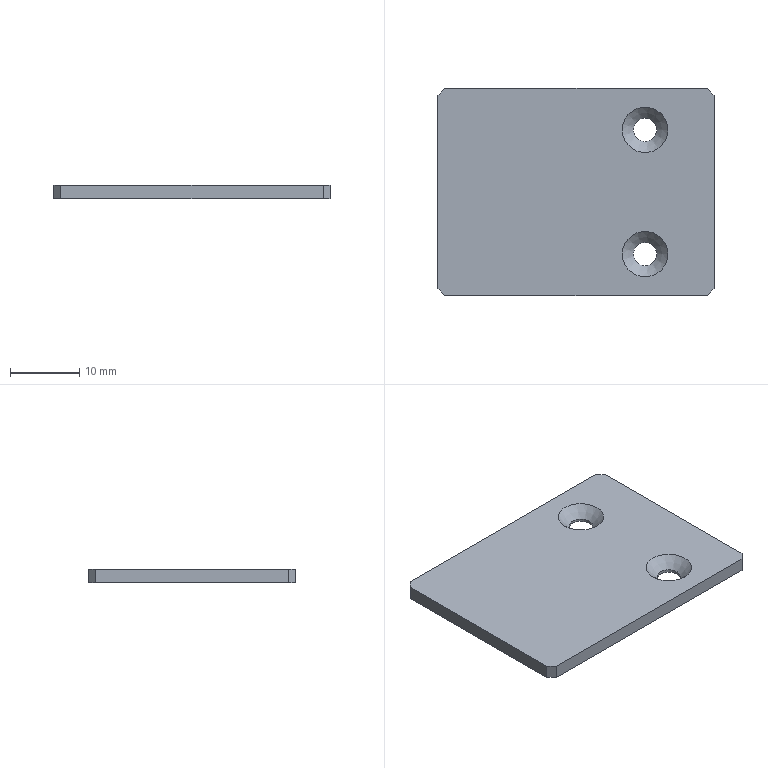Part | NX | 1 solid | 14 faces | box 40 x 30 x 2 mm | volume 2324 mm3 | plane 10 | cylinder 2 | cone 2 | commonest cylinder face diameters 3.4 x2
STEP:
#1=CARTESIAN_POINT('',(-20.,14.,-2.));
#2=VERTEX_POINT('',#1);
#3=CARTESIAN_POINT('',(-20.,-14.,-2.));
#4=VERTEX_POINT('',#3);
#5=CARTESIAN_POINT('',(-20.,-15.,-2.));
#6=DIRECTION('',(0.,-1.,0.));
#7=VECTOR('',#6,1000.);
#8=LINE('',#5,#7);
#9=EDGE_CURVE('',#2,#4,#8,.T.);
#10=ORIENTED_EDGE('',*,*,#9,.T.);
#11=CARTESIAN_POINT('',(-20.,-14.,0.));
#12=VERTEX_POINT('',#11);
#13=CARTESIAN_POINT('',(-20.,-14.,-2.));
#14=DIRECTION('',(0.,0.,1.));
#15=VECTOR('',#14,1000.);
#16=LINE('',#13,#15);
#17=EDGE_CURVE('',#4,#12,#16,.T.);
#18=ORIENTED_EDGE('',*,*,#17,.T.);
#19=CARTESIAN_POINT('',(-20.,14.,0.));
#20=VERTEX_POINT('',#19);
#21=CARTESIAN_POINT('',(-20.,-15.,0.));
#22=DIRECTION('',(0.,-1.,0.));
#23=VECTOR('',#22,1000.);
#24=LINE('',#21,#23);
#25=EDGE_CURVE('',#20,#12,#24,.T.);
#26=ORIENTED_EDGE('',*,*,#25,.F.);
#27=CARTESIAN_POINT('',(-20.,14.,-2.));
#28=DIRECTION('',(0.,0.,-1.));
#29=VECTOR('',#28,1000.);
#30=LINE('',#27,#29);
#31=EDGE_CURVE('',#20,#2,#30,.T.);
#32=ORIENTED_EDGE('',*,*,#31,.T.);
#33=EDGE_LOOP('',(#10,#18,#26,#32));
#34=FACE_BOUND('',#33,.T.);
#35=CARTESIAN_POINT('',(-20.,-15.,-2.));
#36=DIRECTION('',(-1.,0.,0.));
#37=DIRECTION('',(0.,0.,1.));
#38=AXIS2_PLACEMENT_3D('',#35,#36,#37);
#39=PLANE('',#38);
#40=ADVANCED_FACE('',(#34),#39,.T.);
#41=CARTESIAN_POINT('',(19.,15.,0.));
#42=VERTEX_POINT('',#41);
#43=CARTESIAN_POINT('',(-19.,15.,0.));
#44=VERTEX_POINT('',#43);
#45=CARTESIAN_POINT('',(20.,15.,0.));
#46=DIRECTION('',(-1.,0.,0.));
#47=VECTOR('',#46,1000.);
#48=LINE('',#45,#47);
#49=EDGE_CURVE('',#42,#44,#48,.T.);
#50=ORIENTED_EDGE('',*,*,#49,.F.);
#51=CARTESIAN_POINT('',(19.,15.,-2.));
#52=VERTEX_POINT('',#51);
#53=CARTESIAN_POINT('',(19.,15.,-2.));
#54=DIRECTION('',(0.,0.,-1.));
#55=VECTOR('',#54,1000.);
#56=LINE('',#53,#55);
#57=EDGE_CURVE('',#42,#52,#56,.T.);
#58=ORIENTED_EDGE('',*,*,#57,.T.);
#59=CARTESIAN_POINT('',(-19.,15.,-2.));
#60=VERTEX_POINT('',#59);
#61=CARTESIAN_POINT('',(20.,15.,-2.));
#62=DIRECTION('',(-1.,0.,0.));
#63=VECTOR('',#62,1000.);
#64=LINE('',#61,#63);
#65=EDGE_CURVE('',#52,#60,#64,.T.);
#66=ORIENTED_EDGE('',*,*,#65,.T.);
#67=CARTESIAN_POINT('',(-19.,15.,-2.));
#68=DIRECTION('',(0.,0.,1.));
#69=VECTOR('',#68,1000.);
#70=LINE('',#67,#69);
#71=EDGE_CURVE('',#60,#44,#70,.T.);
#72=ORIENTED_EDGE('',*,*,#71,.T.);
#73=EDGE_LOOP('',(#50,#58,#66,#72));
#74=FACE_BOUND('',#73,.T.);
#75=CARTESIAN_POINT('',(20.,15.,-2.));
#76=DIRECTION('',(0.,1.,0.));
#77=DIRECTION('',(-1.,0.,0.));
#78=AXIS2_PLACEMENT_3D('',#75,#76,#77);
#79=PLANE('',#78);
#80=ADVANCED_FACE('',(#74),#79,.T.);
#81=CARTESIAN_POINT('',(20.,-14.,-2.));
#82=VERTEX_POINT('',#81);
#83=CARTESIAN_POINT('',(20.,14.,-2.));
#84=VERTEX_POINT('',#83);
#85=CARTESIAN_POINT('',(20.,-15.,-2.));
#86=DIRECTION('',(0.,1.,0.));
#87=VECTOR('',#86,1000.);
#88=LINE('',#85,#87);
#89=EDGE_CURVE('',#82,#84,#88,.T.);
#90=ORIENTED_EDGE('',*,*,#89,.T.);
#91=CARTESIAN_POINT('',(20.,14.,0.));
#92=VERTEX_POINT('',#91);
#93=CARTESIAN_POINT('',(20.,14.,-2.));
#94=DIRECTION('',(0.,0.,1.));
#95=VECTOR('',#94,1000.);
#96=LINE('',#93,#95);
#97=EDGE_CURVE('',#84,#92,#96,.T.);
#98=ORIENTED_EDGE('',*,*,#97,.T.);
#99=CARTESIAN_POINT('',(20.,-14.,0.));
#100=VERTEX_POINT('',#99);
#101=CARTESIAN_POINT('',(20.,-15.,0.));
#102=DIRECTION('',(0.,1.,0.));
#103=VECTOR('',#102,1000.);
#104=LINE('',#101,#103);
#105=EDGE_CURVE('',#100,#92,#104,.T.);
#106=ORIENTED_EDGE('',*,*,#105,.F.);
#107=CARTESIAN_POINT('',(20.,-14.,-2.));
#108=DIRECTION('',(0.,0.,-1.));
#109=VECTOR('',#108,1000.);
#110=LINE('',#107,#109);
#111=EDGE_CURVE('',#100,#82,#110,.T.);
#112=ORIENTED_EDGE('',*,*,#111,.T.);
#113=EDGE_LOOP('',(#90,#98,#106,#112));
#114=FACE_BOUND('',#113,.T.);
#115=CARTESIAN_POINT('',(20.,-15.,-2.));
#116=DIRECTION('',(1.,0.,0.));
#117=DIRECTION('',(0.,0.,-1.));
#118=AXIS2_PLACEMENT_3D('',#115,#116,#117);
#119=PLANE('',#118);
#120=ADVANCED_FACE('',(#114),#119,.T.);
#121=CARTESIAN_POINT('',(-19.,-15.,-2.));
#122=VERTEX_POINT('',#121);
#123=CARTESIAN_POINT('',(19.,-15.,-2.));
#124=VERTEX_POINT('',#123);
#125=CARTESIAN_POINT('',(20.,-15.,-2.));
#126=DIRECTION('',(1.,0.,0.));
#127=VECTOR('',#126,1000.);
#128=LINE('',#125,#127);
#129=EDGE_CURVE('',#122,#124,#128,.T.);
#130=ORIENTED_EDGE('',*,*,#129,.T.);
#131=CARTESIAN_POINT('',(19.,-15.,0.));
#132=VERTEX_POINT('',#131);
#133=CARTESIAN_POINT('',(19.,-15.,-2.));
#134=DIRECTION('',(0.,0.,1.));
#135=VECTOR('',#134,1000.);
#136=LINE('',#133,#135);
#137=EDGE_CURVE('',#124,#132,#136,.T.);
#138=ORIENTED_EDGE('',*,*,#137,.T.);
#139=CARTESIAN_POINT('',(-19.,-15.,0.));
#140=VERTEX_POINT('',#139);
#141=CARTESIAN_POINT('',(20.,-15.,0.));
#142=DIRECTION('',(1.,0.,0.));
#143=VECTOR('',#142,1000.);
#144=LINE('',#141,#143);
#145=EDGE_CURVE('',#140,#132,#144,.T.);
#146=ORIENTED_EDGE('',*,*,#145,.F.);
#147=CARTESIAN_POINT('',(-19.,-15.,-2.));
#148=DIRECTION('',(0.,0.,-1.));
#149=VECTOR('',#148,1000.);
#150=LINE('',#147,#149);
#151=EDGE_CURVE('',#140,#122,#150,.T.);
#152=ORIENTED_EDGE('',*,*,#151,.T.);
#153=EDGE_LOOP('',(#130,#138,#146,#152));
#154=FACE_BOUND('',#153,.T.);
#155=CARTESIAN_POINT('',(20.,-15.,-2.));
#156=DIRECTION('',(0.,-1.,0.));
#157=DIRECTION('',(1.,0.,0.));
#158=AXIS2_PLACEMENT_3D('',#155,#156,#157);
#159=PLANE('',#158);
#160=ADVANCED_FACE('',(#154),#159,.T.);
#161=CARTESIAN_POINT('',(11.7,9.,-2.));
#162=VERTEX_POINT('',#161);
#163=CARTESIAN_POINT('',(10.,9.,-2.));
#164=DIRECTION('',(0.,0.,1.));
#165=DIRECTION('',(1.,0.,0.));
#166=AXIS2_PLACEMENT_3D('',#163,#164,#165);
#167=CIRCLE('',#166,1.7);
#168=EDGE_CURVE('',#162,#162,#167,.T.);
#169=ORIENTED_EDGE('',*,*,#168,.T.);
#170=EDGE_LOOP('',(#169));
#171=FACE_BOUND('',#170,.T.);
#172=CARTESIAN_POINT('',(11.7,-9.,-2.));
#173=VERTEX_POINT('',#172);
#174=CARTESIAN_POINT('',(10.,-9.,-2.));
#175=DIRECTION('',(0.,0.,1.));
#176=DIRECTION('',(1.,0.,0.));
#177=AXIS2_PLACEMENT_3D('',#174,#175,#176);
#178=CIRCLE('',#177,1.7);
#179=EDGE_CURVE('',#173,#173,#178,.T.);
#180=ORIENTED_EDGE('',*,*,#179,.T.);
#181=EDGE_LOOP('',(#180));
#182=FACE_BOUND('',#181,.T.);
#183=ORIENTED_EDGE('',*,*,#65,.F.);
#184=CARTESIAN_POINT('',(20.,14.,-2.));
#185=DIRECTION('',(-0.7071,0.7071,0.));
#186=VECTOR('',#185,1000.);
#187=LINE('',#184,#186);
#188=EDGE_CURVE('',#52,#84,#187,.F.);
#189=ORIENTED_EDGE('',*,*,#188,.T.);
#190=ORIENTED_EDGE('',*,*,#89,.F.);
#191=CARTESIAN_POINT('',(19.,-15.,-2.));
#192=DIRECTION('',(0.7071,0.7071,0.));
#193=VECTOR('',#192,1000.);
#194=LINE('',#191,#193);
#195=EDGE_CURVE('',#82,#124,#194,.F.);
#196=ORIENTED_EDGE('',*,*,#195,.T.);
#197=ORIENTED_EDGE('',*,*,#129,.F.);
#198=CARTESIAN_POINT('',(-20.,-14.,-2.));
#199=DIRECTION('',(0.7071,-0.7071,0.));
#200=VECTOR('',#199,1000.);
#201=LINE('',#198,#200);
#202=EDGE_CURVE('',#122,#4,#201,.F.);
#203=ORIENTED_EDGE('',*,*,#202,.T.);
#204=ORIENTED_EDGE('',*,*,#9,.F.);
#205=CARTESIAN_POINT('',(-19.,15.,-2.));
#206=DIRECTION('',(-0.7071,-0.7071,0.));
#207=VECTOR('',#206,1000.);
#208=LINE('',#205,#207);
#209=EDGE_CURVE('',#2,#60,#208,.F.);
#210=ORIENTED_EDGE('',*,*,#209,.T.);
#211=EDGE_LOOP('',(#183,#189,#190,#196,#197,#203,#204,#210));
#212=FACE_BOUND('',#211,.T.);
#213=CARTESIAN_POINT('',(0.,0.,-2.));
#214=DIRECTION('',(0.,0.,1.));
#215=DIRECTION('',(1.,0.,0.));
#216=AXIS2_PLACEMENT_3D('',#213,#214,#215);
#217=PLANE('',#216);
#218=ADVANCED_FACE('',(#171,#182,#212),#217,.F.);
#219=CARTESIAN_POINT('',(13.3,9.,0.));
#220=VERTEX_POINT('',#219);
#221=CARTESIAN_POINT('',(10.,9.,0.));
#222=DIRECTION('',(0.,0.,1.));
#223=DIRECTION('',(1.,0.,0.));
#224=AXIS2_PLACEMENT_3D('',#221,#222,#223);
#225=CIRCLE('',#224,3.3);
#226=EDGE_CURVE('',#220,#220,#225,.T.);
#227=ORIENTED_EDGE('',*,*,#226,.F.);
#228=EDGE_LOOP('',(#227));
#229=FACE_BOUND('',#228,.T.);
#230=CARTESIAN_POINT('',(13.3,-9.,0.));
#231=VERTEX_POINT('',#230);
#232=CARTESIAN_POINT('',(10.,-9.,0.));
#233=DIRECTION('',(0.,0.,1.));
#234=DIRECTION('',(1.,0.,0.));
#235=AXIS2_PLACEMENT_3D('',#232,#233,#234);
#236=CIRCLE('',#235,3.3);
#237=EDGE_CURVE('',#231,#231,#236,.T.);
#238=ORIENTED_EDGE('',*,*,#237,.F.);
#239=EDGE_LOOP('',(#238));
#240=FACE_BOUND('',#239,.T.);
#241=ORIENTED_EDGE('',*,*,#105,.T.);
#242=CARTESIAN_POINT('',(17.,17.,0.));
#243=DIRECTION('',(0.7071,-0.7071,0.));
#244=VECTOR('',#243,1000.);
#245=LINE('',#242,#244);
#246=EDGE_CURVE('',#92,#42,#245,.F.);
#247=ORIENTED_EDGE('',*,*,#246,.T.);
#248=ORIENTED_EDGE('',*,*,#49,.T.);
#249=CARTESIAN_POINT('',(-17.,17.,0.));
#250=DIRECTION('',(0.7071,0.7071,0.));
#251=VECTOR('',#250,1000.);
#252=LINE('',#249,#251);
#253=EDGE_CURVE('',#44,#20,#252,.F.);
#254=ORIENTED_EDGE('',*,*,#253,.T.);
#255=ORIENTED_EDGE('',*,*,#25,.T.);
#256=CARTESIAN_POINT('',(-17.,-17.,0.));
#257=DIRECTION('',(-0.7071,0.7071,0.));
#258=VECTOR('',#257,1000.);
#259=LINE('',#256,#258);
#260=EDGE_CURVE('',#12,#140,#259,.F.);
#261=ORIENTED_EDGE('',*,*,#260,.T.);
#262=ORIENTED_EDGE('',*,*,#145,.T.);
#263=CARTESIAN_POINT('',(17.,-17.,0.));
#264=DIRECTION('',(-0.7071,-0.7071,0.));
#265=VECTOR('',#264,1000.);
#266=LINE('',#263,#265);
#267=EDGE_CURVE('',#132,#100,#266,.F.);
#268=ORIENTED_EDGE('',*,*,#267,.T.);
#269=EDGE_LOOP('',(#241,#247,#248,#254,#255,#261,#262,#268));
#270=FACE_BOUND('',#269,.T.);
#271=CARTESIAN_POINT('',(0.,0.,0.));
#272=DIRECTION('',(0.,0.,1.));
#273=DIRECTION('',(1.,0.,0.));
#274=AXIS2_PLACEMENT_3D('',#271,#272,#273);
#275=PLANE('',#274);
#276=ADVANCED_FACE('',(#229,#240,#270),#275,.T.);
#277=ORIENTED_EDGE('',*,*,#179,.F.);
#278=EDGE_LOOP('',(#277));
#279=FACE_BOUND('',#278,.T.);
#280=CARTESIAN_POINT('',(11.7,-9.,-1.6));
#281=VERTEX_POINT('',#280);
#282=CARTESIAN_POINT('',(10.,-9.,-1.6));
#283=DIRECTION('',(0.,0.,1.));
#284=DIRECTION('',(1.,0.,0.));
#285=AXIS2_PLACEMENT_3D('',#282,#283,#284);
#286=CIRCLE('',#285,1.7);
#287=EDGE_CURVE('',#281,#281,#286,.T.);
#288=ORIENTED_EDGE('',*,*,#287,.T.);
#289=EDGE_LOOP('',(#288));
#290=FACE_BOUND('',#289,.T.);
#291=CARTESIAN_POINT('',(10.,-9.,0.));
#292=DIRECTION('',(0.,0.,1.));
#293=DIRECTION('',(1.,0.,0.));
#294=AXIS2_PLACEMENT_3D('',#291,#292,#293);
#295=CYLINDRICAL_SURFACE('',#294,1.7);
#296=ADVANCED_FACE('',(#279,#290),#295,.F.);
#297=ORIENTED_EDGE('',*,*,#287,.F.);
#298=EDGE_LOOP('',(#297));
#299=FACE_BOUND('',#298,.T.);
#300=ORIENTED_EDGE('',*,*,#237,.T.);
#301=EDGE_LOOP('',(#300));
#302=FACE_BOUND('',#301,.T.);
#303=CARTESIAN_POINT('',(10.,-9.,0.));
#304=DIRECTION('',(0.,0.,1.));
#305=DIRECTION('',(1.,0.,0.));
#306=AXIS2_PLACEMENT_3D('',#303,#304,#305);
#307=CONICAL_SURFACE('',#306,3.3,0.7854);
#308=ADVANCED_FACE('',(#299,#302),#307,.F.);
#309=ORIENTED_EDGE('',*,*,#168,.F.);
#310=EDGE_LOOP('',(#309));
#311=FACE_BOUND('',#310,.T.);
#312=CARTESIAN_POINT('',(11.7,9.,-1.6));
#313=VERTEX_POINT('',#312);
#314=CARTESIAN_POINT('',(10.,9.,-1.6));
#315=DIRECTION('',(0.,0.,1.));
#316=DIRECTION('',(1.,0.,0.));
#317=AXIS2_PLACEMENT_3D('',#314,#315,#316);
#318=CIRCLE('',#317,1.7);
#319=EDGE_CURVE('',#313,#313,#318,.T.);
#320=ORIENTED_EDGE('',*,*,#319,.T.);
#321=EDGE_LOOP('',(#320));
#322=FACE_BOUND('',#321,.T.);
#323=CARTESIAN_POINT('',(10.,9.,0.));
#324=DIRECTION('',(0.,0.,1.));
#325=DIRECTION('',(1.,0.,0.));
#326=AXIS2_PLACEMENT_3D('',#323,#324,#325);
#327=CYLINDRICAL_SURFACE('',#326,1.7);
#328=ADVANCED_FACE('',(#311,#322),#327,.F.);
#329=ORIENTED_EDGE('',*,*,#319,.F.);
#330=EDGE_LOOP('',(#329));
#331=FACE_BOUND('',#330,.T.);
#332=ORIENTED_EDGE('',*,*,#226,.T.);
#333=EDGE_LOOP('',(#332));
#334=FACE_BOUND('',#333,.T.);
#335=CARTESIAN_POINT('',(10.,9.,0.));
#336=DIRECTION('',(0.,0.,1.));
#337=DIRECTION('',(1.,0.,0.));
#338=AXIS2_PLACEMENT_3D('',#335,#336,#337);
#339=CONICAL_SURFACE('',#338,3.3,0.7854);
#340=ADVANCED_FACE('',(#331,#334),#339,.F.);
#341=ORIENTED_EDGE('',*,*,#188,.F.);
#342=ORIENTED_EDGE('',*,*,#57,.F.);
#343=ORIENTED_EDGE('',*,*,#246,.F.);
#344=ORIENTED_EDGE('',*,*,#97,.F.);
#345=EDGE_LOOP('',(#341,#342,#343,#344));
#346=FACE_BOUND('',#345,.T.);
#347=CARTESIAN_POINT('',(20.,14.,-2.));
#348=DIRECTION('',(-0.7071,-0.7071,0.));
#349=DIRECTION('',(0.,0.,1.));
#350=AXIS2_PLACEMENT_3D('',#347,#348,#349);
#351=PLANE('',#350);
#352=ADVANCED_FACE('',(#346),#351,.F.);
#353=ORIENTED_EDGE('',*,*,#195,.F.);
#354=ORIENTED_EDGE('',*,*,#111,.F.);
#355=ORIENTED_EDGE('',*,*,#267,.F.);
#356=ORIENTED_EDGE('',*,*,#137,.F.);
#357=EDGE_LOOP('',(#353,#354,#355,#356));
#358=FACE_BOUND('',#357,.T.);
#359=CARTESIAN_POINT('',(19.,-15.,-2.));
#360=DIRECTION('',(-0.7071,0.7071,0.));
#361=DIRECTION('',(0.,0.,1.));
#362=AXIS2_PLACEMENT_3D('',#359,#360,#361);
#363=PLANE('',#362);
#364=ADVANCED_FACE('',(#358),#363,.F.);
#365=ORIENTED_EDGE('',*,*,#202,.F.);
#366=ORIENTED_EDGE('',*,*,#151,.F.);
#367=ORIENTED_EDGE('',*,*,#260,.F.);
#368=ORIENTED_EDGE('',*,*,#17,.F.);
#369=EDGE_LOOP('',(#365,#366,#367,#368));
#370=FACE_BOUND('',#369,.T.);
#371=CARTESIAN_POINT('',(-20.,-14.,-2.));
#372=DIRECTION('',(0.7071,0.7071,0.));
#373=DIRECTION('',(0.,0.,1.));
#374=AXIS2_PLACEMENT_3D('',#371,#372,#373);
#375=PLANE('',#374);
#376=ADVANCED_FACE('',(#370),#375,.F.);
#377=ORIENTED_EDGE('',*,*,#209,.F.);
#378=ORIENTED_EDGE('',*,*,#31,.F.);
#379=ORIENTED_EDGE('',*,*,#253,.F.);
#380=ORIENTED_EDGE('',*,*,#71,.F.);
#381=EDGE_LOOP('',(#377,#378,#379,#380));
#382=FACE_BOUND('',#381,.T.);
#383=CARTESIAN_POINT('',(-19.,15.,-2.));
#384=DIRECTION('',(0.7071,-0.7071,0.));
#385=DIRECTION('',(0.,0.,1.));
#386=AXIS2_PLACEMENT_3D('',#383,#384,#385);
#387=PLANE('',#386);
#388=ADVANCED_FACE('',(#382),#387,.F.);
#389=CLOSED_SHELL('',(#40,#80,#120,#160,#218,#276,#296,#308,#328,#340,#352,#364,#376,#388));
#390=MANIFOLD_SOLID_BREP('',#389);
#391=(LENGTH_UNIT()NAMED_UNIT(*)SI_UNIT(.MILLI.,.METRE.));
#392=UNCERTAINTY_MEASURE_WITH_UNIT(LENGTH_MEASURE(0.00001),#391,'','');
#393=(NAMED_UNIT(*)PLANE_ANGLE_UNIT()SI_UNIT($,.RADIAN.));
#394=(NAMED_UNIT(*)SI_UNIT($,.STERADIAN.)SOLID_ANGLE_UNIT());
#395=(GEOMETRIC_REPRESENTATION_CONTEXT(3)GLOBAL_UNCERTAINTY_ASSIGNED_CONTEXT((#392))GLOBAL_UNIT_ASSIGNED_CONTEXT((#391,#393,#394))REPRESENTATION_CONTEXT('',''));
#396=ADVANCED_BREP_SHAPE_REPRESENTATION('',(#390),#395);